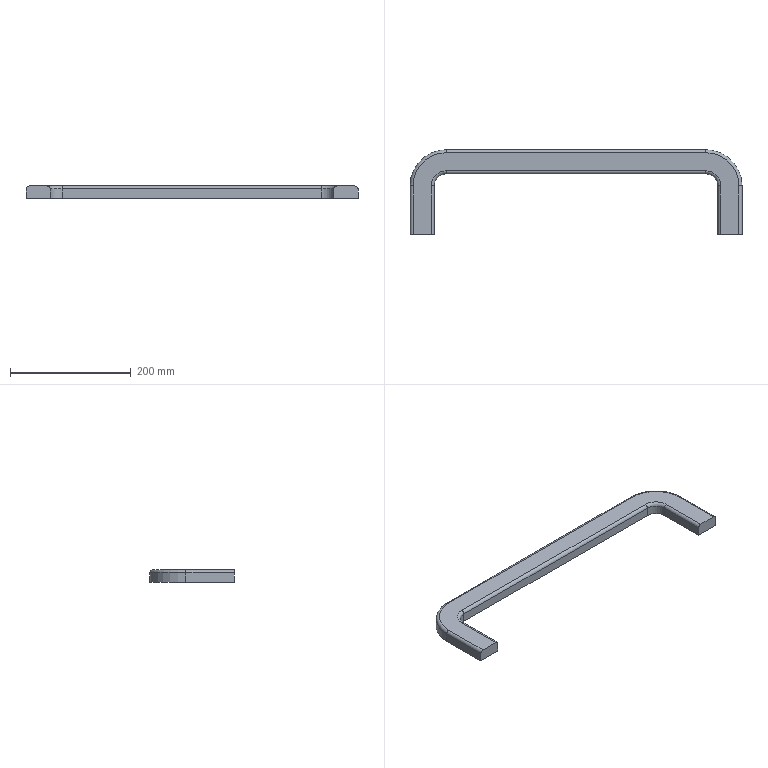Part | SolidWorks | features BaseBody 1 | 1 solid | 24 faces | box 550 x 140 x 20 mm | volume 564852 mm3 | cylinder 10 | plane 10 | torus 4 | commonest cylinder face diameters 10 x6 40 x2 120 x2
STEP:
#1=CARTESIAN_POINT('',(510.,0.,15.));
#2=VERTEX_POINT('',#1);
#3=CARTESIAN_POINT('',(505.,0.,20.));
#4=VERTEX_POINT('',#3);
#5=CARTESIAN_POINT('',(505.,0.,15.));
#6=DIRECTION('',(0.,-1.,0.));
#7=DIRECTION('',(0.,0.,1.));
#8=AXIS2_PLACEMENT_3D('',#5,#6,#7);
#9=CIRCLE('',#8,5.);
#10=EDGE_CURVE('',#2,#4,#9,.T.);
#11=ORIENTED_EDGE('',*,*,#10,.F.);
#12=CARTESIAN_POINT('',(510.,80.,15.));
#13=VERTEX_POINT('',#12);
#14=CARTESIAN_POINT('',(510.,0.,15.));
#15=DIRECTION('',(0.,-1.,0.));
#16=VECTOR('',#15,1000.);
#17=LINE('',#14,#16);
#18=EDGE_CURVE('',#13,#2,#17,.T.);
#19=ORIENTED_EDGE('',*,*,#18,.F.);
#20=CARTESIAN_POINT('',(505.,80.,20.));
#21=VERTEX_POINT('',#20);
#22=CARTESIAN_POINT('',(505.,80.,15.));
#23=DIRECTION('',(0.,-1.,0.));
#24=DIRECTION('',(0.,0.,-1.));
#25=AXIS2_PLACEMENT_3D('',#22,#23,#24);
#26=CIRCLE('',#25,5.);
#27=EDGE_CURVE('',#13,#21,#26,.T.);
#28=ORIENTED_EDGE('',*,*,#27,.T.);
#29=CARTESIAN_POINT('',(505.,80.,20.));
#30=DIRECTION('',(0.,1.,0.));
#31=VECTOR('',#30,1000.);
#32=LINE('',#29,#31);
#33=EDGE_CURVE('',#4,#21,#32,.T.);
#34=ORIENTED_EDGE('',*,*,#33,.F.);
#35=EDGE_LOOP('',(#11,#19,#28,#34));
#36=FACE_OUTER_BOUND('',#35,.T.);
#37=CARTESIAN_POINT('',(505.,80.,15.));
#38=DIRECTION('',(0.,-1.,0.));
#39=DIRECTION('',(0.,0.,-1.));
#40=AXIS2_PLACEMENT_3D('',#37,#38,#39);
#41=CYLINDRICAL_SURFACE('',#40,5.);
#42=ADVANCED_FACE('',(#36),#41,.T.);
#43=CARTESIAN_POINT('',(450.,140.,15.));
#44=VERTEX_POINT('',#43);
#45=CARTESIAN_POINT('',(450.,135.,20.));
#46=VERTEX_POINT('',#45);
#47=CARTESIAN_POINT('',(450.,135.,15.));
#48=DIRECTION('',(1.,0.,0.));
#49=DIRECTION('',(0.,0.,-1.));
#50=AXIS2_PLACEMENT_3D('',#47,#48,#49);
#51=CIRCLE('',#50,5.);
#52=EDGE_CURVE('',#44,#46,#51,.T.);
#53=ORIENTED_EDGE('',*,*,#52,.T.);
#54=CARTESIAN_POINT('',(450.,80.,20.));
#55=DIRECTION('',(0.,0.,1.));
#56=DIRECTION('',(1.,0.,0.));
#57=AXIS2_PLACEMENT_3D('',#54,#55,#56);
#58=CIRCLE('',#57,55.);
#59=EDGE_CURVE('',#21,#46,#58,.T.);
#60=ORIENTED_EDGE('',*,*,#59,.F.);
#61=ORIENTED_EDGE('',*,*,#27,.F.);
#62=CARTESIAN_POINT('',(450.,80.,15.));
#63=DIRECTION('',(0.,0.,-1.));
#64=DIRECTION('',(1.,0.,0.));
#65=AXIS2_PLACEMENT_3D('',#62,#63,#64);
#66=CIRCLE('',#65,60.);
#67=EDGE_CURVE('',#44,#13,#66,.T.);
#68=ORIENTED_EDGE('',*,*,#67,.F.);
#69=EDGE_LOOP('',(#53,#60,#61,#68));
#70=FACE_OUTER_BOUND('',#69,.T.);
#71=CARTESIAN_POINT('',(450.,80.,15.));
#72=DIRECTION('',(0.,0.,1.));
#73=DIRECTION('',(1.,0.,0.));
#74=AXIS2_PLACEMENT_3D('',#71,#72,#73);
#75=TOROIDAL_SURFACE('',#74,55.,5.);
#76=ADVANCED_FACE('',(#70),#75,.T.);
#77=CARTESIAN_POINT('',(20.,140.,15.));
#78=VERTEX_POINT('',#77);
#79=CARTESIAN_POINT('',(20.,135.,20.));
#80=VERTEX_POINT('',#79);
#81=CARTESIAN_POINT('',(20.,135.,15.));
#82=DIRECTION('',(1.,0.,0.));
#83=DIRECTION('',(0.,0.,-1.));
#84=AXIS2_PLACEMENT_3D('',#81,#82,#83);
#85=CIRCLE('',#84,5.);
#86=EDGE_CURVE('',#78,#80,#85,.T.);
#87=ORIENTED_EDGE('',*,*,#86,.T.);
#88=CARTESIAN_POINT('',(20.,135.,20.));
#89=DIRECTION('',(-1.,0.,0.));
#90=VECTOR('',#89,1000.);
#91=LINE('',#88,#90);
#92=EDGE_CURVE('',#46,#80,#91,.T.);
#93=ORIENTED_EDGE('',*,*,#92,.F.);
#94=ORIENTED_EDGE('',*,*,#52,.F.);
#95=CARTESIAN_POINT('',(450.,140.,15.));
#96=DIRECTION('',(1.,0.,0.));
#97=VECTOR('',#96,1000.);
#98=LINE('',#95,#97);
#99=EDGE_CURVE('',#78,#44,#98,.T.);
#100=ORIENTED_EDGE('',*,*,#99,.F.);
#101=EDGE_LOOP('',(#87,#93,#94,#100));
#102=FACE_OUTER_BOUND('',#101,.T.);
#103=CARTESIAN_POINT('',(450.,135.,15.));
#104=DIRECTION('',(1.,0.,0.));
#105=DIRECTION('',(0.,0.,-1.));
#106=AXIS2_PLACEMENT_3D('',#103,#104,#105);
#107=CYLINDRICAL_SURFACE('',#106,5.);
#108=ADVANCED_FACE('',(#102),#107,.T.);
#109=CARTESIAN_POINT('',(-40.,80.,15.));
#110=VERTEX_POINT('',#109);
#111=CARTESIAN_POINT('',(-35.,80.,20.));
#112=VERTEX_POINT('',#111);
#113=CARTESIAN_POINT('',(-35.,80.,15.));
#114=DIRECTION('',(0.,1.,0.));
#115=DIRECTION('',(0.,0.,1.));
#116=AXIS2_PLACEMENT_3D('',#113,#114,#115);
#117=CIRCLE('',#116,5.);
#118=EDGE_CURVE('',#110,#112,#117,.T.);
#119=ORIENTED_EDGE('',*,*,#118,.T.);
#120=CARTESIAN_POINT('',(20.,80.,20.));
#121=DIRECTION('',(0.,0.,1.));
#122=DIRECTION('',(1.,0.,0.));
#123=AXIS2_PLACEMENT_3D('',#120,#121,#122);
#124=CIRCLE('',#123,55.);
#125=EDGE_CURVE('',#80,#112,#124,.T.);
#126=ORIENTED_EDGE('',*,*,#125,.F.);
#127=ORIENTED_EDGE('',*,*,#86,.F.);
#128=CARTESIAN_POINT('',(20.,80.,15.));
#129=DIRECTION('',(0.,0.,-1.));
#130=DIRECTION('',(1.,0.,0.));
#131=AXIS2_PLACEMENT_3D('',#128,#129,#130);
#132=CIRCLE('',#131,60.);
#133=EDGE_CURVE('',#110,#78,#132,.T.);
#134=ORIENTED_EDGE('',*,*,#133,.F.);
#135=EDGE_LOOP('',(#119,#126,#127,#134));
#136=FACE_OUTER_BOUND('',#135,.T.);
#137=CARTESIAN_POINT('',(20.,80.,15.));
#138=DIRECTION('',(0.,0.,1.));
#139=DIRECTION('',(1.,0.,0.));
#140=AXIS2_PLACEMENT_3D('',#137,#138,#139);
#141=TOROIDAL_SURFACE('',#140,55.,5.);
#142=ADVANCED_FACE('',(#136),#141,.T.);
#143=CARTESIAN_POINT('',(-35.,0.,20.));
#144=VERTEX_POINT('',#143);
#145=CARTESIAN_POINT('',(-40.,0.,15.));
#146=VERTEX_POINT('',#145);
#147=CARTESIAN_POINT('',(-35.,0.,15.));
#148=DIRECTION('',(0.,-1.,0.));
#149=DIRECTION('',(0.,0.,1.));
#150=AXIS2_PLACEMENT_3D('',#147,#148,#149);
#151=CIRCLE('',#150,5.);
#152=EDGE_CURVE('',#144,#146,#151,.T.);
#153=ORIENTED_EDGE('',*,*,#152,.F.);
#154=CARTESIAN_POINT('',(-35.,0.,20.));
#155=DIRECTION('',(0.,-1.,0.));
#156=VECTOR('',#155,1000.);
#157=LINE('',#154,#156);
#158=EDGE_CURVE('',#112,#144,#157,.T.);
#159=ORIENTED_EDGE('',*,*,#158,.F.);
#160=ORIENTED_EDGE('',*,*,#118,.F.);
#161=CARTESIAN_POINT('',(-40.,80.,15.));
#162=DIRECTION('',(0.,1.,0.));
#163=VECTOR('',#162,1000.);
#164=LINE('',#161,#163);
#165=EDGE_CURVE('',#146,#110,#164,.T.);
#166=ORIENTED_EDGE('',*,*,#165,.F.);
#167=EDGE_LOOP('',(#153,#159,#160,#166));
#168=FACE_OUTER_BOUND('',#167,.T.);
#169=CARTESIAN_POINT('',(-35.,80.,15.));
#170=DIRECTION('',(0.,1.,0.));
#171=DIRECTION('',(0.,0.,1.));
#172=AXIS2_PLACEMENT_3D('',#169,#170,#171);
#173=CYLINDRICAL_SURFACE('',#172,5.);
#174=ADVANCED_FACE('',(#168),#173,.T.);
#175=CARTESIAN_POINT('',(475.,80.,20.));
#176=VERTEX_POINT('',#175);
#177=CARTESIAN_POINT('',(470.,80.,15.));
#178=VERTEX_POINT('',#177);
#179=CARTESIAN_POINT('',(475.,80.,15.));
#180=DIRECTION('',(0.,-1.,0.));
#181=DIRECTION('',(0.,0.,-1.));
#182=AXIS2_PLACEMENT_3D('',#179,#180,#181);
#183=CIRCLE('',#182,5.);
#184=EDGE_CURVE('',#176,#178,#183,.T.);
#185=ORIENTED_EDGE('',*,*,#184,.T.);
#186=CARTESIAN_POINT('',(470.,0.,15.));
#187=VERTEX_POINT('',#186);
#188=CARTESIAN_POINT('',(470.,80.,15.));
#189=DIRECTION('',(0.,1.,0.));
#190=VECTOR('',#189,1000.);
#191=LINE('',#188,#190);
#192=EDGE_CURVE('',#187,#178,#191,.T.);
#193=ORIENTED_EDGE('',*,*,#192,.F.);
#194=CARTESIAN_POINT('',(475.,0.,20.));
#195=VERTEX_POINT('',#194);
#196=CARTESIAN_POINT('',(475.,0.,15.));
#197=DIRECTION('',(0.,-1.,0.));
#198=DIRECTION('',(0.,0.,1.));
#199=AXIS2_PLACEMENT_3D('',#196,#197,#198);
#200=CIRCLE('',#199,5.);
#201=EDGE_CURVE('',#195,#187,#200,.T.);
#202=ORIENTED_EDGE('',*,*,#201,.F.);
#203=CARTESIAN_POINT('',(475.,0.,20.));
#204=DIRECTION('',(0.,-1.,0.));
#205=VECTOR('',#204,1000.);
#206=LINE('',#203,#205);
#207=EDGE_CURVE('',#176,#195,#206,.T.);
#208=ORIENTED_EDGE('',*,*,#207,.F.);
#209=EDGE_LOOP('',(#185,#193,#202,#208));
#210=FACE_OUTER_BOUND('',#209,.T.);
#211=CARTESIAN_POINT('',(475.,80.,15.));
#212=DIRECTION('',(0.,1.,0.));
#213=DIRECTION('',(0.,0.,1.));
#214=AXIS2_PLACEMENT_3D('',#211,#212,#213);
#215=CYLINDRICAL_SURFACE('',#214,5.);
#216=ADVANCED_FACE('',(#210),#215,.T.);
#217=CARTESIAN_POINT('',(450.,105.,20.));
#218=VERTEX_POINT('',#217);
#219=CARTESIAN_POINT('',(450.,100.,15.));
#220=VERTEX_POINT('',#219);
#221=CARTESIAN_POINT('',(450.,105.,15.));
#222=DIRECTION('',(1.,0.,0.));
#223=DIRECTION('',(0.,0.,-1.));
#224=AXIS2_PLACEMENT_3D('',#221,#222,#223);
#225=CIRCLE('',#224,5.);
#226=EDGE_CURVE('',#218,#220,#225,.T.);
#227=ORIENTED_EDGE('',*,*,#226,.T.);
#228=CARTESIAN_POINT('',(450.,80.,15.));
#229=DIRECTION('',(0.,0.,1.));
#230=DIRECTION('',(1.,0.,0.));
#231=AXIS2_PLACEMENT_3D('',#228,#229,#230);
#232=CIRCLE('',#231,20.);
#233=EDGE_CURVE('',#178,#220,#232,.T.);
#234=ORIENTED_EDGE('',*,*,#233,.F.);
#235=ORIENTED_EDGE('',*,*,#184,.F.);
#236=CARTESIAN_POINT('',(450.,80.,20.));
#237=DIRECTION('',(0.,0.,-1.));
#238=DIRECTION('',(1.,0.,0.));
#239=AXIS2_PLACEMENT_3D('',#236,#237,#238);
#240=CIRCLE('',#239,25.);
#241=EDGE_CURVE('',#218,#176,#240,.T.);
#242=ORIENTED_EDGE('',*,*,#241,.F.);
#243=EDGE_LOOP('',(#227,#234,#235,#242));
#244=FACE_OUTER_BOUND('',#243,.T.);
#245=CARTESIAN_POINT('',(450.,80.,15.));
#246=DIRECTION('',(0.,0.,1.));
#247=DIRECTION('',(1.,0.,0.));
#248=AXIS2_PLACEMENT_3D('',#245,#246,#247);
#249=TOROIDAL_SURFACE('',#248,25.,5.);
#250=ADVANCED_FACE('',(#244),#249,.T.);
#251=CARTESIAN_POINT('',(20.,105.,20.));
#252=VERTEX_POINT('',#251);
#253=CARTESIAN_POINT('',(20.,100.,15.));
#254=VERTEX_POINT('',#253);
#255=CARTESIAN_POINT('',(20.,105.,15.));
#256=DIRECTION('',(1.,0.,0.));
#257=DIRECTION('',(0.,0.,-1.));
#258=AXIS2_PLACEMENT_3D('',#255,#256,#257);
#259=CIRCLE('',#258,5.);
#260=EDGE_CURVE('',#252,#254,#259,.T.);
#261=ORIENTED_EDGE('',*,*,#260,.T.);
#262=CARTESIAN_POINT('',(20.,100.,15.));
#263=DIRECTION('',(-1.,0.,0.));
#264=VECTOR('',#263,1000.);
#265=LINE('',#262,#264);
#266=EDGE_CURVE('',#220,#254,#265,.T.);
#267=ORIENTED_EDGE('',*,*,#266,.F.);
#268=ORIENTED_EDGE('',*,*,#226,.F.);
#269=CARTESIAN_POINT('',(450.,105.,20.));
#270=DIRECTION('',(1.,0.,0.));
#271=VECTOR('',#270,1000.);
#272=LINE('',#269,#271);
#273=EDGE_CURVE('',#252,#218,#272,.T.);
#274=ORIENTED_EDGE('',*,*,#273,.F.);
#275=EDGE_LOOP('',(#261,#267,#268,#274));
#276=FACE_OUTER_BOUND('',#275,.T.);
#277=CARTESIAN_POINT('',(450.,105.,15.));
#278=DIRECTION('',(-1.,0.,0.));
#279=DIRECTION('',(0.,0.,1.));
#280=AXIS2_PLACEMENT_3D('',#277,#278,#279);
#281=CYLINDRICAL_SURFACE('',#280,5.);
#282=ADVANCED_FACE('',(#276),#281,.T.);
#283=CARTESIAN_POINT('',(-5.,80.,20.));
#284=VERTEX_POINT('',#283);
#285=CARTESIAN_POINT('',(0.,80.,15.));
#286=VERTEX_POINT('',#285);
#287=CARTESIAN_POINT('',(-5.,80.,15.));
#288=DIRECTION('',(0.,1.,0.));
#289=DIRECTION('',(0.,0.,1.));
#290=AXIS2_PLACEMENT_3D('',#287,#288,#289);
#291=CIRCLE('',#290,5.);
#292=EDGE_CURVE('',#284,#286,#291,.T.);
#293=ORIENTED_EDGE('',*,*,#292,.T.);
#294=CARTESIAN_POINT('',(20.,80.,15.));
#295=DIRECTION('',(0.,0.,1.));
#296=DIRECTION('',(1.,0.,0.));
#297=AXIS2_PLACEMENT_3D('',#294,#295,#296);
#298=CIRCLE('',#297,20.);
#299=EDGE_CURVE('',#254,#286,#298,.T.);
#300=ORIENTED_EDGE('',*,*,#299,.F.);
#301=ORIENTED_EDGE('',*,*,#260,.F.);
#302=CARTESIAN_POINT('',(20.,80.,20.));
#303=DIRECTION('',(0.,0.,-1.));
#304=DIRECTION('',(1.,0.,0.));
#305=AXIS2_PLACEMENT_3D('',#302,#303,#304);
#306=CIRCLE('',#305,25.);
#307=EDGE_CURVE('',#284,#252,#306,.T.);
#308=ORIENTED_EDGE('',*,*,#307,.F.);
#309=EDGE_LOOP('',(#293,#300,#301,#308));
#310=FACE_OUTER_BOUND('',#309,.T.);
#311=CARTESIAN_POINT('',(20.,80.,15.));
#312=DIRECTION('',(0.,0.,1.));
#313=DIRECTION('',(1.,0.,0.));
#314=AXIS2_PLACEMENT_3D('',#311,#312,#313);
#315=TOROIDAL_SURFACE('',#314,25.,5.);
#316=ADVANCED_FACE('',(#310),#315,.T.);
#317=CARTESIAN_POINT('',(0.,0.,15.));
#318=VERTEX_POINT('',#317);
#319=CARTESIAN_POINT('',(-5.,0.,20.));
#320=VERTEX_POINT('',#319);
#321=CARTESIAN_POINT('',(-5.,0.,15.));
#322=DIRECTION('',(0.,-1.,0.));
#323=DIRECTION('',(0.,0.,1.));
#324=AXIS2_PLACEMENT_3D('',#321,#322,#323);
#325=CIRCLE('',#324,5.);
#326=EDGE_CURVE('',#318,#320,#325,.T.);
#327=ORIENTED_EDGE('',*,*,#326,.F.);
#328=CARTESIAN_POINT('',(0.,0.,15.));
#329=DIRECTION('',(0.,-1.,0.));
#330=VECTOR('',#329,1000.);
#331=LINE('',#328,#330);
#332=EDGE_CURVE('',#286,#318,#331,.T.);
#333=ORIENTED_EDGE('',*,*,#332,.F.);
#334=ORIENTED_EDGE('',*,*,#292,.F.);
#335=CARTESIAN_POINT('',(-5.,80.,20.));
#336=DIRECTION('',(0.,1.,0.));
#337=VECTOR('',#336,1000.);
#338=LINE('',#335,#337);
#339=EDGE_CURVE('',#320,#284,#338,.T.);
#340=ORIENTED_EDGE('',*,*,#339,.F.);
#341=EDGE_LOOP('',(#327,#333,#334,#340));
#342=FACE_OUTER_BOUND('',#341,.T.);
#343=CARTESIAN_POINT('',(-5.,80.,15.));
#344=DIRECTION('',(0.,-1.,0.));
#345=DIRECTION('',(0.,0.,-1.));
#346=AXIS2_PLACEMENT_3D('',#343,#344,#345);
#347=CYLINDRICAL_SURFACE('',#346,5.);
#348=ADVANCED_FACE('',(#342),#347,.T.);
#349=CARTESIAN_POINT('',(470.,0.,0.));
#350=VERTEX_POINT('',#349);
#351=CARTESIAN_POINT('',(510.,0.,0.));
#352=VERTEX_POINT('',#351);
#353=CARTESIAN_POINT('',(470.,0.,0.));
#354=DIRECTION('',(1.,0.,0.));
#355=VECTOR('',#354,1000.);
#356=LINE('',#353,#355);
#357=EDGE_CURVE('',#350,#352,#356,.T.);
#358=ORIENTED_EDGE('',*,*,#357,.F.);
#359=CARTESIAN_POINT('',(470.,80.,0.));
#360=VERTEX_POINT('',#359);
#361=CARTESIAN_POINT('',(470.,0.,0.));
#362=DIRECTION('',(0.,-1.,0.));
#363=VECTOR('',#362,1000.);
#364=LINE('',#361,#363);
#365=EDGE_CURVE('',#360,#350,#364,.T.);
#366=ORIENTED_EDGE('',*,*,#365,.F.);
#367=CARTESIAN_POINT('',(450.,100.,0.));
#368=VERTEX_POINT('',#367);
#369=CARTESIAN_POINT('',(450.,80.,0.));
#370=DIRECTION('',(0.,0.,-1.));
#371=DIRECTION('',(1.,0.,0.));
#372=AXIS2_PLACEMENT_3D('',#369,#370,#371);
#373=CIRCLE('',#372,20.);
#374=EDGE_CURVE('',#368,#360,#373,.T.);
#375=ORIENTED_EDGE('',*,*,#374,.F.);
#376=CARTESIAN_POINT('',(20.,100.,0.));
#377=VERTEX_POINT('',#376);
#378=CARTESIAN_POINT('',(450.,100.,0.));
#379=DIRECTION('',(1.,0.,0.));
#380=VECTOR('',#379,1000.);
#381=LINE('',#378,#380);
#382=EDGE_CURVE('',#377,#368,#381,.T.);
#383=ORIENTED_EDGE('',*,*,#382,.F.);
#384=CARTESIAN_POINT('',(0.,80.,0.));
#385=VERTEX_POINT('',#384);
#386=CARTESIAN_POINT('',(20.,80.,0.));
#387=DIRECTION('',(0.,0.,-1.));
#388=DIRECTION('',(1.,0.,0.));
#389=AXIS2_PLACEMENT_3D('',#386,#387,#388);
#390=CIRCLE('',#389,20.);
#391=EDGE_CURVE('',#385,#377,#390,.T.);
#392=ORIENTED_EDGE('',*,*,#391,.F.);
#393=CARTESIAN_POINT('',(0.,0.,0.));
#394=VERTEX_POINT('',#393);
#395=CARTESIAN_POINT('',(0.,80.,0.));
#396=DIRECTION('',(0.,1.,0.));
#397=VECTOR('',#396,1000.);
#398=LINE('',#395,#397);
#399=EDGE_CURVE('',#394,#385,#398,.T.);
#400=ORIENTED_EDGE('',*,*,#399,.F.);
#401=CARTESIAN_POINT('',(-40.,0.,0.));
#402=VERTEX_POINT('',#401);
#403=CARTESIAN_POINT('',(-40.,0.,0.));
#404=DIRECTION('',(1.,0.,0.));
#405=VECTOR('',#404,1000.);
#406=LINE('',#403,#405);
#407=EDGE_CURVE('',#402,#394,#406,.T.);
#408=ORIENTED_EDGE('',*,*,#407,.F.);
#409=CARTESIAN_POINT('',(-40.,80.,0.));
#410=VERTEX_POINT('',#409);
#411=CARTESIAN_POINT('',(-40.,80.,0.));
#412=DIRECTION('',(0.,-1.,0.));
#413=VECTOR('',#412,1000.);
#414=LINE('',#411,#413);
#415=EDGE_CURVE('',#410,#402,#414,.T.);
#416=ORIENTED_EDGE('',*,*,#415,.F.);
#417=CARTESIAN_POINT('',(20.,140.,0.));
#418=VERTEX_POINT('',#417);
#419=CARTESIAN_POINT('',(20.,80.,0.));
#420=DIRECTION('',(0.,0.,1.));
#421=DIRECTION('',(1.,0.,0.));
#422=AXIS2_PLACEMENT_3D('',#419,#420,#421);
#423=CIRCLE('',#422,60.);
#424=EDGE_CURVE('',#418,#410,#423,.T.);
#425=ORIENTED_EDGE('',*,*,#424,.F.);
#426=CARTESIAN_POINT('',(450.,140.,0.));
#427=VERTEX_POINT('',#426);
#428=CARTESIAN_POINT('',(450.,140.,0.));
#429=DIRECTION('',(-1.,0.,0.));
#430=VECTOR('',#429,1000.);
#431=LINE('',#428,#430);
#432=EDGE_CURVE('',#427,#418,#431,.T.);
#433=ORIENTED_EDGE('',*,*,#432,.F.);
#434=CARTESIAN_POINT('',(510.,80.,0.));
#435=VERTEX_POINT('',#434);
#436=CARTESIAN_POINT('',(450.,80.,0.));
#437=DIRECTION('',(0.,0.,1.));
#438=DIRECTION('',(1.,0.,0.));
#439=AXIS2_PLACEMENT_3D('',#436,#437,#438);
#440=CIRCLE('',#439,60.);
#441=EDGE_CURVE('',#435,#427,#440,.T.);
#442=ORIENTED_EDGE('',*,*,#441,.F.);
#443=CARTESIAN_POINT('',(510.,0.,0.));
#444=DIRECTION('',(0.,1.,0.));
#445=VECTOR('',#444,1000.);
#446=LINE('',#443,#445);
#447=EDGE_CURVE('',#352,#435,#446,.T.);
#448=ORIENTED_EDGE('',*,*,#447,.F.);
#449=EDGE_LOOP('',(#358,#366,#375,#383,#392,#400,#408,#416,#425,#433,#442,#448));
#450=FACE_OUTER_BOUND('',#449,.T.);
#451=CARTESIAN_POINT('',(450.,80.,0.));
#452=DIRECTION('',(0.,0.,1.));
#453=DIRECTION('',(1.,0.,0.));
#454=AXIS2_PLACEMENT_3D('',#451,#452,#453);
#455=PLANE('',#454);
#456=ADVANCED_FACE('',(#450),#455,.F.);
#457=ORIENTED_EDGE('',*,*,#241,.T.);
#458=ORIENTED_EDGE('',*,*,#207,.T.);
#459=CARTESIAN_POINT('',(470.,0.,20.));
#460=DIRECTION('',(1.,0.,0.));
#461=VECTOR('',#460,1000.);
#462=LINE('',#459,#461);
#463=EDGE_CURVE('',#195,#4,#462,.T.);
#464=ORIENTED_EDGE('',*,*,#463,.T.);
#465=ORIENTED_EDGE('',*,*,#33,.T.);
#466=ORIENTED_EDGE('',*,*,#59,.T.);
#467=ORIENTED_EDGE('',*,*,#92,.T.);
#468=ORIENTED_EDGE('',*,*,#125,.T.);
#469=ORIENTED_EDGE('',*,*,#158,.T.);
#470=CARTESIAN_POINT('',(-40.,0.,20.));
#471=DIRECTION('',(1.,0.,0.));
#472=VECTOR('',#471,1000.);
#473=LINE('',#470,#472);
#474=EDGE_CURVE('',#144,#320,#473,.T.);
#475=ORIENTED_EDGE('',*,*,#474,.T.);
#476=ORIENTED_EDGE('',*,*,#339,.T.);
#477=ORIENTED_EDGE('',*,*,#307,.T.);
#478=ORIENTED_EDGE('',*,*,#273,.T.);
#479=EDGE_LOOP('',(#457,#458,#464,#465,#466,#467,#468,#469,#475,#476,#477,#478));
#480=FACE_OUTER_BOUND('',#479,.T.);
#481=CARTESIAN_POINT('',(450.,80.,20.));
#482=DIRECTION('',(0.,0.,1.));
#483=DIRECTION('',(1.,0.,0.));
#484=AXIS2_PLACEMENT_3D('',#481,#482,#483);
#485=PLANE('',#484);
#486=ADVANCED_FACE('',(#480),#485,.T.);
#487=CARTESIAN_POINT('',(470.,0.,20.));
#488=DIRECTION('',(0.,0.,-1.));
#489=VECTOR('',#488,1000.);
#490=LINE('',#487,#489);
#491=EDGE_CURVE('',#187,#350,#490,.T.);
#492=ORIENTED_EDGE('',*,*,#491,.F.);
#493=ORIENTED_EDGE('',*,*,#192,.T.);
#494=CARTESIAN_POINT('',(470.,80.,20.));
#495=DIRECTION('',(0.,0.,-1.));
#496=VECTOR('',#495,1000.);
#497=LINE('',#494,#496);
#498=EDGE_CURVE('',#178,#360,#497,.T.);
#499=ORIENTED_EDGE('',*,*,#498,.T.);
#500=ORIENTED_EDGE('',*,*,#365,.T.);
#501=EDGE_LOOP('',(#492,#493,#499,#500));
#502=FACE_OUTER_BOUND('',#501,.T.);
#503=CARTESIAN_POINT('',(470.,0.,20.));
#504=DIRECTION('',(1.,0.,0.));
#505=DIRECTION('',(0.,1.,0.));
#506=AXIS2_PLACEMENT_3D('',#503,#504,#505);
#507=PLANE('',#506);
#508=ADVANCED_FACE('',(#502),#507,.F.);
#509=ORIENTED_EDGE('',*,*,#498,.F.);
#510=ORIENTED_EDGE('',*,*,#233,.T.);
#511=CARTESIAN_POINT('',(450.,100.,20.));
#512=DIRECTION('',(0.,0.,-1.));
#513=VECTOR('',#512,1000.);
#514=LINE('',#511,#513);
#515=EDGE_CURVE('',#220,#368,#514,.T.);
#516=ORIENTED_EDGE('',*,*,#515,.T.);
#517=ORIENTED_EDGE('',*,*,#374,.T.);
#518=EDGE_LOOP('',(#509,#510,#516,#517));
#519=FACE_OUTER_BOUND('',#518,.T.);
#520=CARTESIAN_POINT('',(450.,80.,20.));
#521=DIRECTION('',(0.,0.,-1.));
#522=DIRECTION('',(-1.,0.,0.));
#523=AXIS2_PLACEMENT_3D('',#520,#521,#522);
#524=CYLINDRICAL_SURFACE('',#523,20.);
#525=ADVANCED_FACE('',(#519),#524,.F.);
#526=ORIENTED_EDGE('',*,*,#515,.F.);
#527=ORIENTED_EDGE('',*,*,#266,.T.);
#528=CARTESIAN_POINT('',(20.,100.,20.));
#529=DIRECTION('',(0.,0.,-1.));
#530=VECTOR('',#529,1000.);
#531=LINE('',#528,#530);
#532=EDGE_CURVE('',#254,#377,#531,.T.);
#533=ORIENTED_EDGE('',*,*,#532,.T.);
#534=ORIENTED_EDGE('',*,*,#382,.T.);
#535=EDGE_LOOP('',(#526,#527,#533,#534));
#536=FACE_OUTER_BOUND('',#535,.T.);
#537=CARTESIAN_POINT('',(450.,100.,20.));
#538=DIRECTION('',(0.,1.,0.));
#539=DIRECTION('',(1.,0.,0.));
#540=AXIS2_PLACEMENT_3D('',#537,#538,#539);
#541=PLANE('',#540);
#542=ADVANCED_FACE('',(#536),#541,.F.);
#543=ORIENTED_EDGE('',*,*,#532,.F.);
#544=ORIENTED_EDGE('',*,*,#299,.T.);
#545=CARTESIAN_POINT('',(0.,80.,20.));
#546=DIRECTION('',(0.,0.,-1.));
#547=VECTOR('',#546,1000.);
#548=LINE('',#545,#547);
#549=EDGE_CURVE('',#286,#385,#548,.T.);
#550=ORIENTED_EDGE('',*,*,#549,.T.);
#551=ORIENTED_EDGE('',*,*,#391,.T.);
#552=EDGE_LOOP('',(#543,#544,#550,#551));
#553=FACE_OUTER_BOUND('',#552,.T.);
#554=CARTESIAN_POINT('',(20.,80.,20.));
#555=DIRECTION('',(0.,0.,-1.));
#556=DIRECTION('',(-1.,0.,0.));
#557=AXIS2_PLACEMENT_3D('',#554,#555,#556);
#558=CYLINDRICAL_SURFACE('',#557,20.);
#559=ADVANCED_FACE('',(#553),#558,.F.);
#560=ORIENTED_EDGE('',*,*,#549,.F.);
#561=ORIENTED_EDGE('',*,*,#332,.T.);
#562=CARTESIAN_POINT('',(0.,0.,20.));
#563=DIRECTION('',(0.,0.,-1.));
#564=VECTOR('',#563,1000.);
#565=LINE('',#562,#564);
#566=EDGE_CURVE('',#318,#394,#565,.T.);
#567=ORIENTED_EDGE('',*,*,#566,.T.);
#568=ORIENTED_EDGE('',*,*,#399,.T.);
#569=EDGE_LOOP('',(#560,#561,#567,#568));
#570=FACE_OUTER_BOUND('',#569,.T.);
#571=CARTESIAN_POINT('',(0.,80.,20.));
#572=DIRECTION('',(-1.,0.,0.));
#573=DIRECTION('',(0.,0.,1.));
#574=AXIS2_PLACEMENT_3D('',#571,#572,#573);
#575=PLANE('',#574);
#576=ADVANCED_FACE('',(#570),#575,.F.);
#577=ORIENTED_EDGE('',*,*,#566,.F.);
#578=ORIENTED_EDGE('',*,*,#326,.T.);
#579=ORIENTED_EDGE('',*,*,#474,.F.);
#580=ORIENTED_EDGE('',*,*,#152,.T.);
#581=CARTESIAN_POINT('',(-40.,0.,20.));
#582=DIRECTION('',(0.,0.,-1.));
#583=VECTOR('',#582,1000.);
#584=LINE('',#581,#583);
#585=EDGE_CURVE('',#146,#402,#584,.T.);
#586=ORIENTED_EDGE('',*,*,#585,.T.);
#587=ORIENTED_EDGE('',*,*,#407,.T.);
#588=EDGE_LOOP('',(#577,#578,#579,#580,#586,#587));
#589=FACE_OUTER_BOUND('',#588,.T.);
#590=CARTESIAN_POINT('',(-40.,0.,20.));
#591=DIRECTION('',(0.,1.,0.));
#592=DIRECTION('',(1.,0.,0.));
#593=AXIS2_PLACEMENT_3D('',#590,#591,#592);
#594=PLANE('',#593);
#595=ADVANCED_FACE('',(#589),#594,.F.);
#596=ORIENTED_EDGE('',*,*,#585,.F.);
#597=ORIENTED_EDGE('',*,*,#165,.T.);
#598=CARTESIAN_POINT('',(-40.,80.,20.));
#599=DIRECTION('',(0.,0.,-1.));
#600=VECTOR('',#599,1000.);
#601=LINE('',#598,#600);
#602=EDGE_CURVE('',#110,#410,#601,.T.);
#603=ORIENTED_EDGE('',*,*,#602,.T.);
#604=ORIENTED_EDGE('',*,*,#415,.T.);
#605=EDGE_LOOP('',(#596,#597,#603,#604));
#606=FACE_OUTER_BOUND('',#605,.T.);
#607=CARTESIAN_POINT('',(-40.,80.,20.));
#608=DIRECTION('',(1.,0.,0.));
#609=DIRECTION('',(0.,1.,0.));
#610=AXIS2_PLACEMENT_3D('',#607,#608,#609);
#611=PLANE('',#610);
#612=ADVANCED_FACE('',(#606),#611,.F.);
#613=ORIENTED_EDGE('',*,*,#602,.F.);
#614=ORIENTED_EDGE('',*,*,#133,.T.);
#615=CARTESIAN_POINT('',(20.,140.,20.));
#616=DIRECTION('',(0.,0.,-1.));
#617=VECTOR('',#616,1000.);
#618=LINE('',#615,#617);
#619=EDGE_CURVE('',#78,#418,#618,.T.);
#620=ORIENTED_EDGE('',*,*,#619,.T.);
#621=ORIENTED_EDGE('',*,*,#424,.T.);
#622=EDGE_LOOP('',(#613,#614,#620,#621));
#623=FACE_OUTER_BOUND('',#622,.T.);
#624=CARTESIAN_POINT('',(20.,80.,20.));
#625=DIRECTION('',(0.,0.,-1.));
#626=DIRECTION('',(-1.,0.,0.));
#627=AXIS2_PLACEMENT_3D('',#624,#625,#626);
#628=CYLINDRICAL_SURFACE('',#627,60.);
#629=ADVANCED_FACE('',(#623),#628,.T.);
#630=ORIENTED_EDGE('',*,*,#619,.F.);
#631=ORIENTED_EDGE('',*,*,#99,.T.);
#632=CARTESIAN_POINT('',(450.,140.,20.));
#633=DIRECTION('',(0.,0.,-1.));
#634=VECTOR('',#633,1000.);
#635=LINE('',#632,#634);
#636=EDGE_CURVE('',#44,#427,#635,.T.);
#637=ORIENTED_EDGE('',*,*,#636,.T.);
#638=ORIENTED_EDGE('',*,*,#432,.T.);
#639=EDGE_LOOP('',(#630,#631,#637,#638));
#640=FACE_OUTER_BOUND('',#639,.T.);
#641=CARTESIAN_POINT('',(450.,140.,20.));
#642=DIRECTION('',(0.,-1.,0.));
#643=DIRECTION('',(0.,0.,-1.));
#644=AXIS2_PLACEMENT_3D('',#641,#642,#643);
#645=PLANE('',#644);
#646=ADVANCED_FACE('',(#640),#645,.F.);
#647=ORIENTED_EDGE('',*,*,#636,.F.);
#648=ORIENTED_EDGE('',*,*,#67,.T.);
#649=CARTESIAN_POINT('',(510.,80.,20.));
#650=DIRECTION('',(0.,0.,-1.));
#651=VECTOR('',#650,1000.);
#652=LINE('',#649,#651);
#653=EDGE_CURVE('',#13,#435,#652,.T.);
#654=ORIENTED_EDGE('',*,*,#653,.T.);
#655=ORIENTED_EDGE('',*,*,#441,.T.);
#656=EDGE_LOOP('',(#647,#648,#654,#655));
#657=FACE_OUTER_BOUND('',#656,.T.);
#658=CARTESIAN_POINT('',(450.,80.,20.));
#659=DIRECTION('',(0.,0.,-1.));
#660=DIRECTION('',(-1.,0.,0.));
#661=AXIS2_PLACEMENT_3D('',#658,#659,#660);
#662=CYLINDRICAL_SURFACE('',#661,60.);
#663=ADVANCED_FACE('',(#657),#662,.T.);
#664=ORIENTED_EDGE('',*,*,#653,.F.);
#665=ORIENTED_EDGE('',*,*,#18,.T.);
#666=CARTESIAN_POINT('',(510.,0.,20.));
#667=DIRECTION('',(0.,0.,-1.));
#668=VECTOR('',#667,1000.);
#669=LINE('',#666,#668);
#670=EDGE_CURVE('',#2,#352,#669,.T.);
#671=ORIENTED_EDGE('',*,*,#670,.T.);
#672=ORIENTED_EDGE('',*,*,#447,.T.);
#673=EDGE_LOOP('',(#664,#665,#671,#672));
#674=FACE_OUTER_BOUND('',#673,.T.);
#675=CARTESIAN_POINT('',(510.,0.,20.));
#676=DIRECTION('',(-1.,0.,0.));
#677=DIRECTION('',(0.,0.,1.));
#678=AXIS2_PLACEMENT_3D('',#675,#676,#677);
#679=PLANE('',#678);
#680=ADVANCED_FACE('',(#674),#679,.F.);
#681=ORIENTED_EDGE('',*,*,#463,.F.);
#682=ORIENTED_EDGE('',*,*,#201,.T.);
#683=ORIENTED_EDGE('',*,*,#491,.T.);
#684=ORIENTED_EDGE('',*,*,#357,.T.);
#685=ORIENTED_EDGE('',*,*,#670,.F.);
#686=ORIENTED_EDGE('',*,*,#10,.T.);
#687=EDGE_LOOP('',(#681,#682,#683,#684,#685,#686));
#688=FACE_OUTER_BOUND('',#687,.T.);
#689=CARTESIAN_POINT('',(470.,0.,20.));
#690=DIRECTION('',(0.,1.,0.));
#691=DIRECTION('',(1.,0.,0.));
#692=AXIS2_PLACEMENT_3D('',#689,#690,#691);
#693=PLANE('',#692);
#694=ADVANCED_FACE('',(#688),#693,.F.);
#695=CLOSED_SHELL('',(#42,#76,#108,#142,#174,#216,#250,#282,#316,#348,#456,#486,#508,#525,#542,#559,#576,#595,#612,#629,#646,#663,#680,#694));
#696=MANIFOLD_SOLID_BREP('',#695);
#697=CARTESIAN_POINT('',(0.,0.,0.));
#698=DIRECTION('',(0.,0.,1.));
#699=DIRECTION('',(1.,0.,0.));
#700=AXIS2_PLACEMENT_3D('',#697,#698,#699);
#701=(LENGTH_UNIT()NAMED_UNIT(*)SI_UNIT(.MILLI.,.METRE.));
#702=UNCERTAINTY_MEASURE_WITH_UNIT(LENGTH_MEASURE(0.00001),#701,'','');
#703=(NAMED_UNIT(*)PLANE_ANGLE_UNIT()SI_UNIT($,.RADIAN.));
#704=(NAMED_UNIT(*)SI_UNIT($,.STERADIAN.)SOLID_ANGLE_UNIT());
#705=(GEOMETRIC_REPRESENTATION_CONTEXT(3)GLOBAL_UNCERTAINTY_ASSIGNED_CONTEXT((#702))GLOBAL_UNIT_ASSIGNED_CONTEXT((#701,#703,#704))REPRESENTATION_CONTEXT('',''));
#706=ADVANCED_BREP_SHAPE_REPRESENTATION('',(#696,#700),#705);